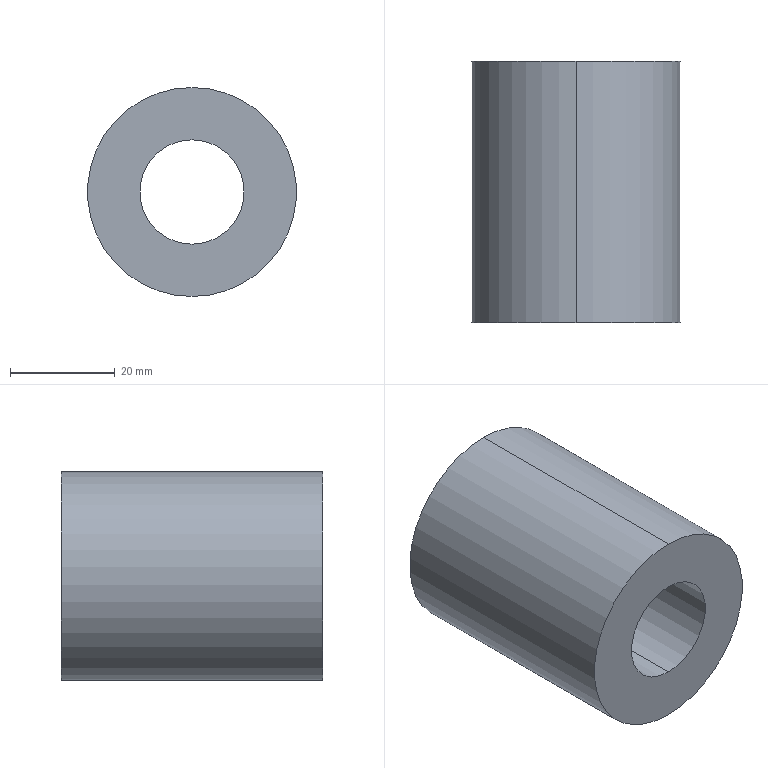Part | SolidWorks | features Extrusion 1 | 1 solid | 6 faces | box 40 x 50 x 40 mm | volume 47124 mm3 | cylinder 4 | plane 2 | commonest cylinder face diameters 20 x2 40 x2
STEP:
#1=CARTESIAN_POINT('',(0.,50.,-10.));
#2=VERTEX_POINT('',#1);
#3=CARTESIAN_POINT('',(0.,50.,10.));
#4=VERTEX_POINT('',#3);
#5=CARTESIAN_POINT('',(0.,50.,0.));
#6=DIRECTION('',(0.,1.,0.));
#7=DIRECTION('',(0.,0.,1.));
#8=AXIS2_PLACEMENT_3D('',#5,#6,#7);
#9=CIRCLE('',#8,10.);
#10=EDGE_CURVE('',#2,#4,#9,.T.);
#11=ORIENTED_EDGE('',*,*,#10,.T.);
#12=CARTESIAN_POINT('',(0.,0.,10.));
#13=VERTEX_POINT('',#12);
#14=CARTESIAN_POINT('',(0.,50.,10.));
#15=DIRECTION('',(0.,-1.,0.));
#16=VECTOR('',#15,1000.);
#17=LINE('',#14,#16);
#18=EDGE_CURVE('',#4,#13,#17,.T.);
#19=ORIENTED_EDGE('',*,*,#18,.T.);
#20=CARTESIAN_POINT('',(0.,0.,-10.));
#21=VERTEX_POINT('',#20);
#22=CARTESIAN_POINT('',(0.,0.,0.));
#23=DIRECTION('',(0.,1.,0.));
#24=DIRECTION('',(0.,0.,1.));
#25=AXIS2_PLACEMENT_3D('',#22,#23,#24);
#26=CIRCLE('',#25,10.);
#27=EDGE_CURVE('',#21,#13,#26,.T.);
#28=ORIENTED_EDGE('',*,*,#27,.F.);
#29=CARTESIAN_POINT('',(0.,50.,-10.));
#30=DIRECTION('',(0.,-1.,0.));
#31=VECTOR('',#30,1000.);
#32=LINE('',#29,#31);
#33=EDGE_CURVE('',#2,#21,#32,.T.);
#34=ORIENTED_EDGE('',*,*,#33,.F.);
#35=EDGE_LOOP('',(#11,#19,#28,#34));
#36=FACE_OUTER_BOUND('',#35,.T.);
#37=CARTESIAN_POINT('',(0.,50.,0.));
#38=DIRECTION('',(0.,-1.,0.));
#39=DIRECTION('',(0.,0.,-1.));
#40=AXIS2_PLACEMENT_3D('',#37,#38,#39);
#41=CYLINDRICAL_SURFACE('',#40,10.);
#42=ADVANCED_FACE('',(#36),#41,.F.);
#43=CARTESIAN_POINT('',(0.,50.,20.));
#44=VERTEX_POINT('',#43);
#45=CARTESIAN_POINT('',(0.,50.,-20.));
#46=VERTEX_POINT('',#45);
#47=CARTESIAN_POINT('',(0.,50.,0.));
#48=DIRECTION('',(0.,1.,0.));
#49=DIRECTION('',(0.,0.,1.));
#50=AXIS2_PLACEMENT_3D('',#47,#48,#49);
#51=CIRCLE('',#50,20.);
#52=EDGE_CURVE('',#44,#46,#51,.T.);
#53=ORIENTED_EDGE('',*,*,#52,.F.);
#54=CARTESIAN_POINT('',(0.,0.,20.));
#55=VERTEX_POINT('',#54);
#56=CARTESIAN_POINT('',(0.,50.,20.));
#57=DIRECTION('',(0.,-1.,0.));
#58=VECTOR('',#57,1000.);
#59=LINE('',#56,#58);
#60=EDGE_CURVE('',#44,#55,#59,.T.);
#61=ORIENTED_EDGE('',*,*,#60,.T.);
#62=CARTESIAN_POINT('',(0.,0.,-20.));
#63=VERTEX_POINT('',#62);
#64=CARTESIAN_POINT('',(0.,0.,0.));
#65=DIRECTION('',(0.,1.,0.));
#66=DIRECTION('',(0.,0.,1.));
#67=AXIS2_PLACEMENT_3D('',#64,#65,#66);
#68=CIRCLE('',#67,20.);
#69=EDGE_CURVE('',#55,#63,#68,.T.);
#70=ORIENTED_EDGE('',*,*,#69,.T.);
#71=CARTESIAN_POINT('',(0.,50.,-20.));
#72=DIRECTION('',(0.,-1.,0.));
#73=VECTOR('',#72,1000.);
#74=LINE('',#71,#73);
#75=EDGE_CURVE('',#46,#63,#74,.T.);
#76=ORIENTED_EDGE('',*,*,#75,.F.);
#77=EDGE_LOOP('',(#53,#61,#70,#76));
#78=FACE_OUTER_BOUND('',#77,.T.);
#79=CARTESIAN_POINT('',(0.,50.,0.));
#80=DIRECTION('',(0.,-1.,0.));
#81=DIRECTION('',(0.,0.,-1.));
#82=AXIS2_PLACEMENT_3D('',#79,#80,#81);
#83=CYLINDRICAL_SURFACE('',#82,20.);
#84=ADVANCED_FACE('',(#78),#83,.T.);
#85=CARTESIAN_POINT('',(0.,50.,0.));
#86=DIRECTION('',(0.,1.,0.));
#87=DIRECTION('',(0.,0.,1.));
#88=AXIS2_PLACEMENT_3D('',#85,#86,#87);
#89=CIRCLE('',#88,20.);
#90=EDGE_CURVE('',#46,#44,#89,.T.);
#91=ORIENTED_EDGE('',*,*,#90,.T.);
#92=ORIENTED_EDGE('',*,*,#52,.T.);
#93=EDGE_LOOP('',(#91,#92));
#94=FACE_OUTER_BOUND('',#93,.T.);
#95=ORIENTED_EDGE('',*,*,#10,.F.);
#96=CARTESIAN_POINT('',(0.,50.,0.));
#97=DIRECTION('',(0.,1.,0.));
#98=DIRECTION('',(0.,0.,1.));
#99=AXIS2_PLACEMENT_3D('',#96,#97,#98);
#100=CIRCLE('',#99,10.);
#101=EDGE_CURVE('',#4,#2,#100,.T.);
#102=ORIENTED_EDGE('',*,*,#101,.F.);
#103=EDGE_LOOP('',(#95,#102));
#104=FACE_BOUND('',#103,.T.);
#105=CARTESIAN_POINT('',(0.,50.,0.));
#106=DIRECTION('',(0.,1.,0.));
#107=DIRECTION('',(0.,0.,1.));
#108=AXIS2_PLACEMENT_3D('',#105,#106,#107);
#109=PLANE('',#108);
#110=ADVANCED_FACE('',(#94,#104),#109,.T.);
#111=CARTESIAN_POINT('',(0.,0.,0.));
#112=DIRECTION('',(0.,1.,0.));
#113=DIRECTION('',(0.,0.,1.));
#114=AXIS2_PLACEMENT_3D('',#111,#112,#113);
#115=CIRCLE('',#114,20.);
#116=EDGE_CURVE('',#63,#55,#115,.T.);
#117=ORIENTED_EDGE('',*,*,#116,.F.);
#118=ORIENTED_EDGE('',*,*,#69,.F.);
#119=EDGE_LOOP('',(#117,#118));
#120=FACE_OUTER_BOUND('',#119,.T.);
#121=ORIENTED_EDGE('',*,*,#27,.T.);
#122=CARTESIAN_POINT('',(0.,0.,0.));
#123=DIRECTION('',(0.,1.,0.));
#124=DIRECTION('',(0.,0.,1.));
#125=AXIS2_PLACEMENT_3D('',#122,#123,#124);
#126=CIRCLE('',#125,10.);
#127=EDGE_CURVE('',#13,#21,#126,.T.);
#128=ORIENTED_EDGE('',*,*,#127,.T.);
#129=EDGE_LOOP('',(#121,#128));
#130=FACE_BOUND('',#129,.T.);
#131=CARTESIAN_POINT('',(0.,0.,0.));
#132=DIRECTION('',(0.,1.,0.));
#133=DIRECTION('',(0.,0.,1.));
#134=AXIS2_PLACEMENT_3D('',#131,#132,#133);
#135=PLANE('',#134);
#136=ADVANCED_FACE('',(#120,#130),#135,.F.);
#137=ORIENTED_EDGE('',*,*,#60,.F.);
#138=ORIENTED_EDGE('',*,*,#90,.F.);
#139=ORIENTED_EDGE('',*,*,#75,.T.);
#140=ORIENTED_EDGE('',*,*,#116,.T.);
#141=EDGE_LOOP('',(#137,#138,#139,#140));
#142=FACE_OUTER_BOUND('',#141,.T.);
#143=CARTESIAN_POINT('',(0.,50.,0.));
#144=DIRECTION('',(0.,-1.,0.));
#145=DIRECTION('',(0.,0.,-1.));
#146=AXIS2_PLACEMENT_3D('',#143,#144,#145);
#147=CYLINDRICAL_SURFACE('',#146,20.);
#148=ADVANCED_FACE('',(#142),#147,.T.);
#149=ORIENTED_EDGE('',*,*,#18,.F.);
#150=ORIENTED_EDGE('',*,*,#101,.T.);
#151=ORIENTED_EDGE('',*,*,#33,.T.);
#152=ORIENTED_EDGE('',*,*,#127,.F.);
#153=EDGE_LOOP('',(#149,#150,#151,#152));
#154=FACE_OUTER_BOUND('',#153,.T.);
#155=CARTESIAN_POINT('',(0.,50.,0.));
#156=DIRECTION('',(0.,-1.,0.));
#157=DIRECTION('',(0.,0.,-1.));
#158=AXIS2_PLACEMENT_3D('',#155,#156,#157);
#159=CYLINDRICAL_SURFACE('',#158,10.);
#160=ADVANCED_FACE('',(#154),#159,.F.);
#161=CLOSED_SHELL('',(#42,#84,#110,#136,#148,#160));
#162=MANIFOLD_SOLID_BREP('',#161);
#163=CARTESIAN_POINT('',(0.,0.,0.));
#164=DIRECTION('',(0.,0.,1.));
#165=DIRECTION('',(1.,0.,0.));
#166=AXIS2_PLACEMENT_3D('',#163,#164,#165);
#167=(LENGTH_UNIT()NAMED_UNIT(*)SI_UNIT(.MILLI.,.METRE.));
#168=UNCERTAINTY_MEASURE_WITH_UNIT(LENGTH_MEASURE(0.00001),#167,'','');
#169=(NAMED_UNIT(*)PLANE_ANGLE_UNIT()SI_UNIT($,.RADIAN.));
#170=(NAMED_UNIT(*)SI_UNIT($,.STERADIAN.)SOLID_ANGLE_UNIT());
#171=(GEOMETRIC_REPRESENTATION_CONTEXT(3)GLOBAL_UNCERTAINTY_ASSIGNED_CONTEXT((#168))GLOBAL_UNIT_ASSIGNED_CONTEXT((#167,#169,#170))REPRESENTATION_CONTEXT('',''));
#172=ADVANCED_BREP_SHAPE_REPRESENTATION('',(#162,#166),#171);